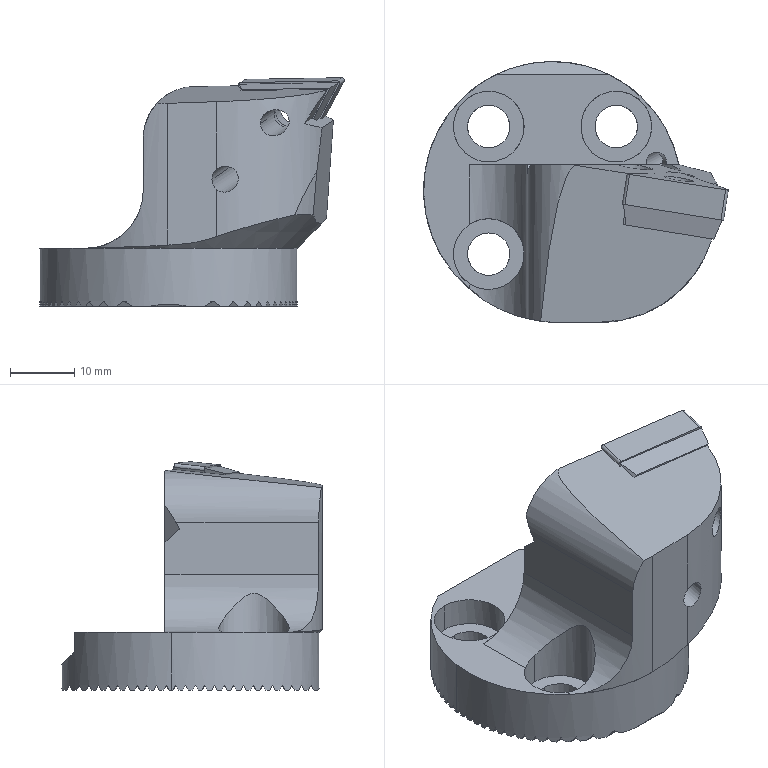NC program | Mastercam | posted with a generic post
Lines 8003 to 9736 of 11065, first 1620 of 1734 lines:
(4 FEMR |TOOL - 6|DIA. OFF. - 6|LEN. - 6|TOOL DIA. - 4.)
N6152 T6 M6
N6154 G0 G54 G90 X26.879 Y19.28 C9. B-84. S3500 M3
N6156 G43 H6 Z58.245
N6158 Z9.245
N6160 G1 Z8.146 F2000.
N6162 G41 D6 X26.556 Y19.863 F500.
N6164 G3 X26.468 Y19.915 I-.088 J-.049
N6166 X26.42 Y19.902 J-.101
N6168 G1 X25.334 Y19.3
N6170 X22.57 Y19.348
N6172 X22.567
N6174 G3 X22.437 Y19.218 J-.13
N6176 X22.565 Y19.088 I.13
N6178 G1 X25.33 Y19.04
N6180 X26.394 Y18.401
N6182 G3 X26.445 Y18.387 I.051 J.086
N6184 X26.531 Y18.435 J.1
N6186 G1 G40 X26.874 Y19.007
N6188 X26.879 Y19.28
N6190 Z8.046 F2000.
N6192 G41 D6 X26.556 Y19.863 F500.
N6194 G3 X26.468 Y19.915 I-.088 J-.049
N6196 X26.42 Y19.902 J-.101
N6198 G1 X25.334 Y19.3
N6200 X22.57 Y19.348
N6202 X22.567
N6204 G3 X22.437 Y19.218 J-.13
N6206 X22.565 Y19.088 I.13
N6208 G1 X25.33 Y19.04
N6210 X26.394 Y18.401
N6212 G3 X26.445 Y18.387 I.051 J.086
N6214 X26.531 Y18.435 J.1
N6216 G1 G40 X26.874 Y19.007
N6218 X26.879 Y19.28
N6220 Z7.947 F2000.
N6222 G41 D6 X26.556 Y19.863 F500.
N6224 G3 X26.468 Y19.915 I-.088 J-.049
N6226 X26.42 Y19.902 J-.101
N6228 G1 X25.334 Y19.3
N6230 X22.57 Y19.348
N6232 X22.567
N6234 G3 X22.437 Y19.218 J-.13
N6236 X22.565 Y19.088 I.13
N6238 G1 X25.33 Y19.04
N6240 X26.394 Y18.401
N6242 G3 X26.445 Y18.387 I.051 J.086
N6244 X26.531 Y18.435 J.1
N6246 G1 G40 X26.874 Y19.007
N6248 X26.879 Y19.28
N6250 Z7.848 F2000.
N6252 G41 D6 X26.556 Y19.863 F500.
N6254 G3 X26.468 Y19.915 I-.088 J-.049
N6256 X26.42 Y19.902 J-.101
N6258 G1 X25.334 Y19.3
N6260 X22.57 Y19.348
N6262 X22.567
N6264 G3 X22.437 Y19.218 J-.13
N6266 X22.565 Y19.088 I.13
N6268 G1 X25.33 Y19.04
N6270 X26.394 Y18.401
N6272 G3 X26.445 Y18.387 I.051 J.086
N6274 X26.531 Y18.435 J.1
N6276 G1 G40 X26.874 Y19.007
N6278 X26.879 Y19.28
N6280 Z7.748 F2000.
N6282 G41 D6 X26.556 Y19.863 F500.
N6284 G3 X26.468 Y19.915 I-.088 J-.049
N6286 X26.42 Y19.902 J-.101
N6288 G1 X25.334 Y19.3
N6290 X22.57 Y19.348
N6292 X22.567
N6294 G3 X22.437 Y19.218 J-.13
N6296 X22.565 Y19.088 I.13
N6298 G1 X25.33 Y19.04
N6300 X26.394 Y18.401
N6302 G3 X26.445 Y18.387 I.051 J.086
N6304 X26.531 Y18.435 J.1
N6306 G1 G40 X26.874 Y19.007
N6308 X26.879 Y19.28
N6310 Z7.649 F2000.
N6312 G41 D6 X26.556 Y19.863 F500.
N6314 G3 X26.468 Y19.915 I-.088 J-.049
N6316 X26.42 Y19.902 J-.101
N6318 G1 X25.334 Y19.3
N6320 X22.57 Y19.348
N6322 X22.567
N6324 G3 X22.437 Y19.218 J-.13
N6326 X22.565 Y19.088 I.13
N6328 G1 X25.33 Y19.04
N6330 X26.394 Y18.401
N6332 G3 X26.445 Y18.387 I.051 J.086
N6334 X26.531 Y18.435 J.1
N6336 G1 G40 X26.874 Y19.007
N6338 X26.879 Y19.28
N6340 Z7.55 F2000.
N6342 G41 D6 X26.556 Y19.863 F500.
N6344 G3 X26.468 Y19.915 I-.088 J-.049
N6346 X26.42 Y19.902 J-.101
N6348 G1 X25.334 Y19.3
N6350 X22.57 Y19.348
N6352 X22.567
N6354 G3 X22.437 Y19.218 J-.13
N6356 X22.565 Y19.088 I.13
N6358 G1 X25.33 Y19.04
N6360 X26.394 Y18.401
N6362 G3 X26.445 Y18.387 I.051 J.086
N6364 X26.531 Y18.435 J.1
N6366 G1 G40 X26.874 Y19.007
N6368 X26.879 Y19.28
N6370 Z7.45 F2000.
N6372 G41 D6 X26.556 Y19.863 F500.
N6374 G3 X26.468 Y19.915 I-.088 J-.049
N6376 X26.42 Y19.902 J-.101
N6378 G1 X25.334 Y19.3
N6380 X22.57 Y19.348
N6382 X22.567
N6384 G3 X22.437 Y19.218 J-.13
N6386 X22.565 Y19.088 I.13
N6388 G1 X25.33 Y19.04
N6390 X26.394 Y18.401
N6392 G3 X26.445 Y18.387 I.051 J.086
N6394 X26.531 Y18.435 J.1
N6396 G1 G40 X26.874 Y19.007
N6398 X26.879 Y19.28
N6400 Z7.351 F2000.
N6402 G41 D6 X26.556 Y19.863 F500.
N6404 G3 X26.468 Y19.915 I-.088 J-.049
N6406 X26.42 Y19.902 J-.101
N6408 G1 X25.334 Y19.3
N6410 X22.57 Y19.348
N6412 X22.567
N6414 G3 X22.437 Y19.218 J-.13
N6416 X22.565 Y19.088 I.13
N6418 G1 X25.33 Y19.04
N6420 X26.394 Y18.401
N6422 G3 X26.445 Y18.387 I.051 J.086
N6424 X26.531 Y18.435 J.1
N6426 G1 G40 X26.874 Y19.007
N6428 X26.879 Y19.28
N6430 Z7.251 F2000.
N6432 G41 D6 X26.556 Y19.863 F500.
N6434 G3 X26.468 Y19.915 I-.088 J-.049
N6436 X26.42 Y19.902 J-.101
N6438 G1 X25.334 Y19.3
N6440 X22.57 Y19.348
N6442 X22.567
N6444 G3 X22.437 Y19.218 J-.13
N6446 X22.565 Y19.088 I.13
N6448 G1 X25.33 Y19.04
N6450 X26.394 Y18.401
N6452 G3 X26.445 Y18.387 I.051 J.086
N6454 X26.531 Y18.435 J.1
N6456 G1 G40 X26.874 Y19.007
N6458 X26.879 Y19.28
N6460 Z7.152 F2000.
N6462 G41 D6 X26.556 Y19.863 F500.
N6464 G3 X26.468 Y19.915 I-.088 J-.049
N6466 X26.42 Y19.902 J-.101
N6468 G1 X25.334 Y19.3
N6470 X22.57 Y19.348
N6472 X22.567
N6474 G3 X22.437 Y19.218 J-.13
N6476 X22.565 Y19.088 I.13
N6478 G1 X25.33 Y19.04
N6480 X26.394 Y18.401
N6482 G3 X26.445 Y18.387 I.051 J.086
N6484 X26.531 Y18.435 J.1
N6486 G1 G40 X26.874 Y19.007
N6488 X26.879 Y19.28
N6490 Z7.053 F2000.
N6492 G41 D6 X26.556 Y19.863 F500.
N6494 G3 X26.468 Y19.915 I-.088 J-.049
N6496 X26.42 Y19.902 J-.101
N6498 G1 X25.334 Y19.3
N6500 X22.57 Y19.348
N6502 X22.567
N6504 G3 X22.437 Y19.218 J-.13
N6506 X22.565 Y19.088 I.13
N6508 G1 X25.33 Y19.04
N6510 X26.394 Y18.401
N6512 G3 X26.445 Y18.387 I.051 J.086
N6514 X26.531 Y18.435 J.1
N6516 G1 G40 X26.874 Y19.007
N6518 X26.879 Y19.28
N6520 Z6.953 F2000.
N6522 G41 D6 X26.556 Y19.863 F500.
N6524 G3 X26.468 Y19.915 I-.088 J-.049
N6526 X26.42 Y19.902 J-.101
N6528 G1 X25.334 Y19.3
N6530 X22.57 Y19.348
N6532 X22.567
N6534 G3 X22.437 Y19.218 J-.13
N6536 X22.565 Y19.088 I.13
N6538 G1 X25.33 Y19.04
N6540 X26.394 Y18.401
N6542 G3 X26.445 Y18.387 I.051 J.086
N6544 X26.531 Y18.435 J.1
N6546 G1 G40 X26.874 Y19.007
N6548 X26.879 Y19.28
N6550 Z6.854 F2000.
N6552 G41 D6 X26.556 Y19.863 F500.
N6554 G3 X26.468 Y19.915 I-.088 J-.049
N6556 X26.42 Y19.902 J-.101
N6558 G1 X25.334 Y19.3
N6560 X22.57 Y19.348
N6562 X22.567
N6564 G3 X22.437 Y19.218 J-.13
N6566 X22.565 Y19.088 I.13
N6568 G1 X25.33 Y19.04
N6570 X26.394 Y18.401
N6572 G3 X26.445 Y18.387 I.051 J.086
N6574 X26.531 Y18.435 J.1
N6576 G1 G40 X26.874 Y19.007
N6578 X26.879 Y19.28
N6580 Z6.754 F2000.
N6582 G41 D6 X26.556 Y19.863 F500.
N6584 G3 X26.468 Y19.915 I-.088 J-.049
N6586 X26.42 Y19.902 J-.101
N6588 G1 X25.334 Y19.3
N6590 X22.57 Y19.348
N6592 X22.567
N6594 G3 X22.437 Y19.218 J-.13
N6596 X22.565 Y19.088 I.13
N6598 G1 X25.33 Y19.04
N6600 X26.394 Y18.401
N6602 G3 X26.445 Y18.387 I.051 J.086
N6604 X26.531 Y18.435 J.1
N6606 G1 G40 X26.874 Y19.007
N6608 X26.879 Y19.28
N6610 Z6.655 F2000.
N6612 G41 D6 X26.556 Y19.863 F500.
N6614 G3 X26.468 Y19.915 I-.088 J-.049
N6616 X26.42 Y19.902 J-.101
N6618 G1 X25.334 Y19.3
N6620 X22.57 Y19.348
N6622 X22.567
N6624 G3 X22.437 Y19.218 J-.13
N6626 X22.565 Y19.088 I.13
N6628 G1 X25.33 Y19.04
N6630 X26.394 Y18.401
N6632 G3 X26.445 Y18.387 I.051 J.086
N6634 X26.531 Y18.435 J.1
N6636 G1 G40 X26.874 Y19.007
N6638 X26.879 Y19.28
N6640 Z6.556 F2000.
N6642 G41 D6 X26.556 Y19.863 F500.
N6644 G3 X26.468 Y19.915 I-.088 J-.049
N6646 X26.42 Y19.902 J-.101
N6648 G1 X25.334 Y19.3
N6650 X22.57 Y19.348
N6652 X22.567
N6654 G3 X22.437 Y19.218 J-.13
N6656 X22.565 Y19.088 I.13
N6658 G1 X25.33 Y19.04
N6660 X26.394 Y18.401
N6662 G3 X26.445 Y18.387 I.051 J.086
N6664 X26.531 Y18.435 J.1
N6666 G1 G40 X26.874 Y19.007
N6668 X26.879 Y19.28
N6670 Z6.456 F2000.
N6672 G41 D6 X26.556 Y19.863 F500.
N6674 G3 X26.468 Y19.915 I-.088 J-.049
N6676 X26.42 Y19.902 J-.101
N6678 G1 X25.334 Y19.3
N6680 X22.57 Y19.348
N6682 X22.567
N6684 G3 X22.437 Y19.218 J-.13
N6686 X22.565 Y19.088 I.13
N6688 G1 X25.33 Y19.04
N6690 X26.394 Y18.401
N6692 G3 X26.445 Y18.387 I.051 J.086
N6694 X26.531 Y18.435 J.1
N6696 G1 G40 X26.874 Y19.007
N6698 X26.879 Y19.28
N6700 Z6.357 F2000.
N6702 G41 D6 X26.556 Y19.863 F500.
N6704 G3 X26.468 Y19.915 I-.088 J-.049
N6706 X26.42 Y19.902 J-.101
N6708 G1 X25.334 Y19.3
N6710 X22.57 Y19.348
N6712 X22.567
N6714 G3 X22.437 Y19.218 J-.13
N6716 X22.565 Y19.088 I.13
N6718 G1 X25.33 Y19.04
N6720 X26.394 Y18.401
N6722 G3 X26.445 Y18.387 I.051 J.086
N6724 X26.531 Y18.435 J.1
N6726 G1 G40 X26.874 Y19.007
N6728 X26.879 Y19.28
N6730 Z6.257 F2000.
N6732 G41 D6 X26.556 Y19.863 F500.
N6734 G3 X26.468 Y19.915 I-.088 J-.049
N6736 X26.42 Y19.902 J-.101
N6738 G1 X25.334 Y19.3
N6740 X22.57 Y19.348
N6742 X22.567
N6744 G3 X22.437 Y19.218 J-.13
N6746 X22.565 Y19.088 I.13
N6748 G1 X25.33 Y19.04
N6750 X26.394 Y18.401
N6752 G3 X26.445 Y18.387 I.051 J.086
N6754 X26.531 Y18.435 J.1
N6756 G1 G40 X26.874 Y19.007
N6758 X26.879 Y19.28
N6760 Z6.158 F2000.
N6762 G41 D6 X26.556 Y19.863 F500.
N6764 G3 X26.468 Y19.915 I-.088 J-.049
N6766 X26.42 Y19.902 J-.101
N6768 G1 X25.334 Y19.3
N6770 X22.57 Y19.348
N6772 X22.567
N6774 G3 X22.437 Y19.218 J-.13
N6776 X22.565 Y19.088 I.13
N6778 G1 X25.33 Y19.04
N6780 X26.394 Y18.401
N6782 G3 X26.445 Y18.387 I.051 J.086
N6784 X26.531 Y18.435 J.1
N6786 G1 G40 X26.874 Y19.007
N6788 X26.879 Y19.28
N6790 Z6.059 F2000.
N6792 G41 D6 X26.556 Y19.863 F500.
N6794 G3 X26.468 Y19.915 I-.088 J-.049
N6796 X26.42 Y19.902 J-.101
N6798 G1 X25.334 Y19.3
N6800 X22.57 Y19.348
N6802 X22.567
N6804 G3 X22.437 Y19.218 J-.13
N6806 X22.565 Y19.088 I.13
N6808 G1 X25.33 Y19.04
N6810 X26.394 Y18.401
N6812 G3 X26.445 Y18.387 I.051 J.086
N6814 X26.531 Y18.435 J.1
N6816 G1 G40 X26.874 Y19.007
N6818 X26.879 Y19.28
N6820 Z5.959 F2000.
N6822 G41 D6 X26.556 Y19.863 F500.
N6824 G3 X26.468 Y19.915 I-.088 J-.049
N6826 X26.42 Y19.902 J-.101
N6828 G1 X25.334 Y19.3
N6830 X22.57 Y19.348
N6832 X22.567
N6834 G3 X22.437 Y19.218 J-.13
N6836 X22.565 Y19.088 I.13
N6838 G1 X25.33 Y19.04
N6840 X26.394 Y18.401
N6842 G3 X26.445 Y18.387 I.051 J.086
N6844 X26.531 Y18.435 J.1
N6846 G1 G40 X26.874 Y19.007
N6848 X26.879 Y19.28
N6850 Z5.86 F2000.
N6852 G41 D6 X26.556 Y19.863 F500.
N6854 G3 X26.468 Y19.915 I-.088 J-.049
N6856 X26.42 Y19.902 J-.101
N6858 G1 X25.334 Y19.3
N6860 X22.57 Y19.348
N6862 X22.567
N6864 G3 X22.437 Y19.218 J-.13
N6866 X22.565 Y19.088 I.13
N6868 G1 X25.33 Y19.04
N6870 X26.394 Y18.401
N6872 G3 X26.445 Y18.387 I.051 J.086
N6874 X26.531 Y18.435 J.1
N6876 G1 G40 X26.874 Y19.007
N6878 X26.879 Y19.28
N6880 Z5.76 F2000.
N6882 G41 D6 X26.556 Y19.863 F500.
N6884 G3 X26.468 Y19.915 I-.088 J-.049
N6886 X26.42 Y19.902 J-.101
N6888 G1 X25.334 Y19.3
N6890 X22.57 Y19.348
N6892 X22.567
N6894 G3 X22.437 Y19.218 J-.13
N6896 X22.565 Y19.088 I.13
N6898 G1 X25.33 Y19.04
N6900 X26.394 Y18.401
N6902 G3 X26.445 Y18.387 I.051 J.086
N6904 X26.531 Y18.435 J.1
N6906 G1 G40 X26.874 Y19.007
N6908 X26.879 Y19.28
N6910 Z5.661 F2000.
N6912 G41 D6 X26.556 Y19.863 F500.
N6914 G3 X26.468 Y19.915 I-.088 J-.049
N6916 X26.42 Y19.902 J-.101
N6918 G1 X25.334 Y19.3
N6920 X22.57 Y19.348
N6922 X22.567
N6924 G3 X22.437 Y19.218 J-.13
N6926 X22.565 Y19.088 I.13
N6928 G1 X25.33 Y19.04
N6930 X26.394 Y18.401
N6932 G3 X26.445 Y18.387 I.051 J.086
N6934 X26.531 Y18.435 J.1
N6936 G1 G40 X26.874 Y19.007
N6938 X26.879 Y19.28
N6940 Z5.562 F2000.
N6942 G41 D6 X26.556 Y19.863 F500.
N6944 G3 X26.468 Y19.915 I-.088 J-.049
N6946 X26.42 Y19.902 J-.101
N6948 G1 X25.334 Y19.3
N6950 X22.57 Y19.348
N6952 X22.567
N6954 G3 X22.437 Y19.218 J-.13
N6956 X22.565 Y19.088 I.13
N6958 G1 X25.33 Y19.04
N6960 X26.394 Y18.401
N6962 G3 X26.445 Y18.387 I.051 J.086
N6964 X26.531 Y18.435 J.1
N6966 G1 G40 X26.874 Y19.007
N6968 X26.879 Y19.28
N6970 Z5.462 F2000.
N6972 G41 D6 X26.556 Y19.863 F500.
N6974 G3 X26.468 Y19.915 I-.088 J-.049
N6976 X26.42 Y19.902 J-.101
N6978 G1 X25.334 Y19.3
N6980 X22.57 Y19.348
N6982 X22.567
N6984 G3 X22.437 Y19.218 J-.13
N6986 X22.565 Y19.088 I.13
N6988 G1 X25.33 Y19.04
N6990 X26.394 Y18.401
N6992 G3 X26.445 Y18.387 I.051 J.086
N6994 X26.531 Y18.435 J.1
N6996 G1 G40 X26.874 Y19.007
N6998 X26.879 Y19.28
N7000 Z5.363 F2000.
N7002 G41 D6 X26.556 Y19.863 F500.
N7004 G3 X26.468 Y19.915 I-.088 J-.049
N7006 X26.42 Y19.902 J-.101
N7008 G1 X25.334 Y19.3
N7010 X22.57 Y19.348
N7012 X22.567
N7014 G3 X22.437 Y19.218 J-.13
N7016 X22.565 Y19.088 I.13
N7018 G1 X25.33 Y19.04
N7020 X26.394 Y18.401
N7022 G3 X26.445 Y18.387 I.051 J.086
N7024 X26.531 Y18.435 J.1
N7026 G1 G40 X26.874 Y19.007
N7028 X26.879 Y19.28
N7030 Z5.263 F2000.
N7032 G41 D6 X26.556 Y19.863 F500.
N7034 G3 X26.468 Y19.915 I-.088 J-.049
N7036 X26.42 Y19.902 J-.101
N7038 G1 X25.334 Y19.3
N7040 X22.57 Y19.348
N7042 X22.567
N7044 G3 X22.437 Y19.218 J-.13
N7046 X22.565 Y19.088 I.13
N7048 G1 X25.33 Y19.04
N7050 X26.394 Y18.401
N7052 G3 X26.445 Y18.387 I.051 J.086
N7054 X26.531 Y18.435 J.1
N7056 G1 G40 X26.874 Y19.007
N7058 X26.879 Y19.28
N7060 Z5.164 F2000.
N7062 G41 D6 X26.556 Y19.863 F500.
N7064 G3 X26.468 Y19.915 I-.088 J-.049
N7066 X26.42 Y19.902 J-.101
N7068 G1 X25.334 Y19.3
N7070 X22.57 Y19.348
N7072 X22.567
N7074 G3 X22.437 Y19.218 J-.13
N7076 X22.565 Y19.088 I.13
N7078 G1 X25.33 Y19.04
N7080 X26.394 Y18.401
N7082 G3 X26.445 Y18.387 I.051 J.086
N7084 X26.531 Y18.435 J.1
N7086 G1 G40 X26.874 Y19.007
N7088 X26.879 Y19.28
N7090 Z5.065 F2000.
N7092 G41 D6 X26.556 Y19.863 F500.
N7094 G3 X26.468 Y19.915 I-.088 J-.049
N7096 X26.42 Y19.902 J-.101
N7098 G1 X25.334 Y19.3
N7100 X22.57 Y19.348
N7102 X22.567
N7104 G3 X22.437 Y19.218 J-.13
N7106 X22.565 Y19.088 I.13
N7108 G1 X25.33 Y19.04
N7110 X26.394 Y18.401
N7112 G3 X26.445 Y18.387 I.051 J.086
N7114 X26.531 Y18.435 J.1
N7116 G1 G40 X26.874 Y19.007
N7118 X26.879 Y19.28
N7120 Z4.965 F2000.
N7122 G41 D6 X26.556 Y19.863 F500.
N7124 G3 X26.468 Y19.915 I-.088 J-.049
N7126 X26.42 Y19.902 J-.101
N7128 G1 X25.334 Y19.3
N7130 X22.57 Y19.348
N7132 X22.567
N7134 G3 X22.437 Y19.218 J-.13
N7136 X22.565 Y19.088 I.13
N7138 G1 X25.33 Y19.04
N7140 X26.394 Y18.401
N7142 G3 X26.445 Y18.387 I.051 J.086
N7144 X26.531 Y18.435 J.1
N7146 G1 G40 X26.874 Y19.007
N7148 X26.879 Y19.28
N7150 Z4.866 F2000.
N7152 G41 D6 X26.556 Y19.863 F500.
N7154 G3 X26.468 Y19.915 I-.088 J-.049
N7156 X26.42 Y19.902 J-.101
N7158 G1 X25.334 Y19.3
N7160 X22.57 Y19.348
N7162 X22.567
N7164 G3 X22.437 Y19.218 J-.13
N7166 X22.565 Y19.088 I.13
N7168 G1 X25.33 Y19.04
N7170 X26.394 Y18.401
N7172 G3 X26.445 Y18.387 I.051 J.086
N7174 X26.531 Y18.435 J.1
N7176 G1 G40 X26.874 Y19.007
N7178 X26.879 Y19.28
N7180 Z4.766 F2000.
N7182 G41 D6 X26.556 Y19.863 F500.
N7184 G3 X26.468 Y19.915 I-.088 J-.049
N7186 X26.42 Y19.902 J-.101
N7188 G1 X25.334 Y19.3
N7190 X22.57 Y19.348
N7192 X22.567
N7194 G3 X22.437 Y19.218 J-.13
N7196 X22.565 Y19.088 I.13
N7198 G1 X25.33 Y19.04
N7200 X26.394 Y18.401
N7202 G3 X26.445 Y18.387 I.051 J.086
N7204 X26.531 Y18.435 J.1
N7206 G1 G40 X26.874 Y19.007
N7208 X26.879 Y19.28
N7210 Z4.667 F2000.
N7212 G41 D6 X26.556 Y19.863 F500.
N7214 G3 X26.468 Y19.915 I-.088 J-.049
N7216 X26.42 Y19.902 J-.101
N7218 G1 X25.334 Y19.3
N7220 X22.57 Y19.348
N7222 X22.567
N7224 G3 X22.437 Y19.218 J-.13
N7226 X22.565 Y19.088 I.13
N7228 G1 X25.33 Y19.04
N7230 X26.394 Y18.401
N7232 G3 X26.445 Y18.387 I.051 J.086
N7234 X26.531 Y18.435 J.1
N7236 G1 G40 X26.874 Y19.007
N7238 X26.879 Y19.28
N7240 Z4.568 F2000.
N7242 G41 D6 X26.556 Y19.863 F500.
N7244 G3 X26.468 Y19.915 I-.088 J-.049
N7246 X26.42 Y19.902 J-.101
N7248 G1 X25.334 Y19.3
N7250 X22.57 Y19.348
N7252 X22.567
N7254 G3 X22.437 Y19.218 J-.13
N7256 X22.565 Y19.088 I.13
N7258 G1 X25.33 Y19.04
N7260 X26.394 Y18.401
N7262 G3 X26.445 Y18.387 I.051 J.086
N7264 X26.531 Y18.435 J.1
N7266 G1 G40 X26.874 Y19.007
N7268 X26.879 Y19.28
N7270 Z4.468 F2000.
N7272 G41 D6 X26.556 Y19.863 F500.
N7274 G3 X26.468 Y19.915 I-.088 J-.049
N7276 X26.42 Y19.902 J-.101
N7278 G1 X25.334 Y19.3
N7280 X22.57 Y19.348
N7282 X22.567
N7284 G3 X22.437 Y19.218 J-.13
N7286 X22.565 Y19.088 I.13
N7288 G1 X25.33 Y19.04
N7290 X26.394 Y18.401
N7292 G3 X26.445 Y18.387 I.051 J.086
N7294 X26.531 Y18.435 J.1
N7296 G1 G40 X26.874 Y19.007
N7298 X26.879 Y19.28
N7300 Z4.369 F2000.
N7302 G41 D6 X26.556 Y19.863 F500.
N7304 G3 X26.468 Y19.915 I-.088 J-.049
N7306 X26.42 Y19.902 J-.101
N7308 G1 X25.334 Y19.3
N7310 X22.57 Y19.348
N7312 X22.567
N7314 G3 X22.437 Y19.218 J-.13
N7316 X22.565 Y19.088 I.13
N7318 G1 X25.33 Y19.04
N7320 X26.394 Y18.401
N7322 G3 X26.445 Y18.387 I.051 J.086
N7324 X26.531 Y18.435 J.1
N7326 G1 G40 X26.874 Y19.007
N7328 X26.879 Y19.28
N7330 Z4.269 F2000.
N7332 G41 D6 X26.556 Y19.863 F500.
N7334 G3 X26.468 Y19.915 I-.088 J-.049
N7336 X26.42 Y19.902 J-.101
N7338 G1 X25.334 Y19.3
N7340 X22.57 Y19.348
N7342 X22.567
N7344 G3 X22.437 Y19.218 J-.13
N7346 X22.565 Y19.088 I.13
N7348 G1 X25.33 Y19.04
N7350 X26.394 Y18.401
N7352 G3 X26.445 Y18.387 I.051 J.086
N7354 X26.531 Y18.435 J.1
N7356 G1 G40 X26.874 Y19.007
N7358 X26.879 Y19.28
N7360 Z4.17 F2000.
N7362 G41 D6 X26.556 Y19.863 F500.
N7364 G3 X26.468 Y19.915 I-.088 J-.049
N7366 X26.42 Y19.902 J-.101
N7368 G1 X25.334 Y19.3
N7370 X22.57 Y19.348
N7372 X22.567
N7374 G3 X22.437 Y19.218 J-.13
N7376 X22.565 Y19.088 I.13
N7378 G1 X25.33 Y19.04
N7380 X26.394 Y18.401
N7382 G3 X26.445 Y18.387 I.051 J.086
N7384 X26.531 Y18.435 J.1
N7386 G1 G40 X26.874 Y19.007
N7388 X26.879 Y19.28
N7390 Z4.071 F2000.
N7392 G41 D6 X26.556 Y19.863 F500.
N7394 G3 X26.468 Y19.915 I-.088 J-.049
N7396 X26.42 Y19.902 J-.101
N7398 G1 X25.334 Y19.3
N7400 X22.57 Y19.348
N7402 X22.567
N7404 G3 X22.437 Y19.218 J-.13
N7406 X22.565 Y19.088 I.13
N7408 G1 X25.33 Y19.04
N7410 X26.394 Y18.401
N7412 G3 X26.445 Y18.387 I.051 J.086
N7414 X26.531 Y18.435 J.1
N7416 G1 G40 X26.874 Y19.007
N7418 X26.879 Y19.28
N7420 Z3.971 F2000.
N7422 G41 D6 X26.556 Y19.863 F500.
N7424 G3 X26.468 Y19.915 I-.088 J-.049
N7426 X26.42 Y19.902 J-.101
N7428 G1 X25.334 Y19.3
N7430 X22.57 Y19.348
N7432 X22.567
N7434 G3 X22.437 Y19.218 J-.13
N7436 X22.565 Y19.088 I.13
N7438 G1 X25.33 Y19.04
N7440 X26.394 Y18.401
N7442 G3 X26.445 Y18.387 I.051 J.086
N7444 X26.531 Y18.435 J.1
N7446 G1 G40 X26.874 Y19.007
N7448 X26.879 Y19.28
N7450 Z3.872 F2000.
N7452 G41 D6 X26.556 Y19.863 F500.
N7454 G3 X26.468 Y19.915 I-.088 J-.049
N7456 X26.42 Y19.902 J-.101
N7458 G1 X25.334 Y19.3
N7460 X22.57 Y19.348
N7462 X22.567
N7464 G3 X22.437 Y19.218 J-.13
N7466 X22.565 Y19.088 I.13
N7468 G1 X25.33 Y19.04
N7470 X26.394 Y18.401
N7472 G3 X26.445 Y18.387 I.051 J.086
N7474 X26.531 Y18.435 J.1
N7476 G1 G40 X26.874 Y19.007
N7478 X26.879 Y19.28
N7480 Z3.772 F2000.
N7482 G41 D6 X26.556 Y19.863 F500.
N7484 G3 X26.468 Y19.915 I-.088 J-.049
N7486 X26.42 Y19.902 J-.101
N7488 G1 X25.334 Y19.3
N7490 X22.57 Y19.348
N7492 X22.567
N7494 G3 X22.437 Y19.218 J-.13
N7496 X22.565 Y19.088 I.13
N7498 G1 X25.33 Y19.04
N7500 X26.394 Y18.401
N7502 G3 X26.445 Y18.387 I.051 J.086
N7504 X26.531 Y18.435 J.1
N7506 G1 G40 X26.874 Y19.007
N7508 X26.879 Y19.28
N7510 Z3.673 F2000.
N7512 G41 D6 X26.556 Y19.863 F500.
N7514 G3 X26.468 Y19.915 I-.088 J-.049
N7516 X26.42 Y19.902 J-.101
N7518 G1 X25.334 Y19.3
N7520 X22.57 Y19.348
N7522 X22.567
N7524 G3 X22.437 Y19.218 J-.13
N7526 X22.565 Y19.088 I.13
N7528 G1 X25.33 Y19.04
N7530 X26.394 Y18.401
N7532 G3 X26.445 Y18.387 I.051 J.086
N7534 X26.531 Y18.435 J.1
N7536 G1 G40 X26.874 Y19.007
N7538 X26.879 Y19.28
N7540 Z3.574 F2000.
N7542 G41 D6 X26.556 Y19.863 F500.
N7544 G3 X26.468 Y19.915 I-.088 J-.049
N7546 X26.42 Y19.902 J-.101
N7548 G1 X25.334 Y19.3
N7550 X22.57 Y19.348
N7552 X22.567
N7554 G3 X22.437 Y19.218 J-.13
N7556 X22.565 Y19.088 I.13
N7558 G1 X25.33 Y19.04
N7560 X26.394 Y18.401
N7562 G3 X26.445 Y18.387 I.051 J.086
N7564 X26.531 Y18.435 J.1
N7566 G1 G40 X26.874 Y19.007
N7568 X26.879 Y19.28
N7570 Z3.474 F2000.
N7572 G41 D6 X26.556 Y19.863 F500.
N7574 G3 X26.468 Y19.915 I-.088 J-.049
N7576 X26.42 Y19.902 J-.101
N7578 G1 X25.334 Y19.3
N7580 X22.57 Y19.348
N7582 X22.567
N7584 G3 X22.437 Y19.218 J-.13
N7586 X22.565 Y19.088 I.13
N7588 G1 X25.33 Y19.04
N7590 X26.394 Y18.401
N7592 G3 X26.445 Y18.387 I.051 J.086
N7594 X26.531 Y18.435 J.1
N7596 G1 G40 X26.874 Y19.007
N7598 X26.879 Y19.28
N7600 Z3.375 F2000.
N7602 G41 D6 X26.556 Y19.863 F500.
N7604 G3 X26.468 Y19.915 I-.088 J-.049
N7606 X26.42 Y19.902 J-.101
N7608 G1 X25.334 Y19.3
N7610 X22.57 Y19.348
N7612 X22.567
N7614 G3 X22.437 Y19.218 J-.13
N7616 X22.565 Y19.088 I.13
N7618 G1 X25.33 Y19.04
N7620 X26.394 Y18.401
N7622 G3 X26.445 Y18.387 I.051 J.086
N7624 X26.531 Y18.435 J.1
N7626 G1 G40 X26.874 Y19.007
N7628 X26.879 Y19.28
N7630 Z3.275 F2000.
N7632 G41 D6 X26.556 Y19.863 F500.
N7634 G3 X26.468 Y19.915 I-.088 J-.049
N7636 X26.42 Y19.902 J-.101
N7638 G1 X25.334 Y19.3
N7640 X22.57 Y19.348
N7642 X22.567
N7644 G3 X22.437 Y19.218 J-.13
N7646 X22.565 Y19.088 I.13
N7648 G1 X25.33 Y19.04
N7650 X26.394 Y18.401
N7652 G3 X26.445 Y18.387 I.051 J.086
N7654 X26.531 Y18.435 J.1
N7656 G1 G40 X26.874 Y19.007
N7658 X26.879 Y19.28
N7660 Z3.176 F2000.
N7662 G41 D6 X26.556 Y19.863 F500.
N7664 G3 X26.468 Y19.915 I-.088 J-.049
N7666 X26.42 Y19.902 J-.101
N7668 G1 X25.334 Y19.3
N7670 X22.57 Y19.348
N7672 X22.567
N7674 G3 X22.437 Y19.218 J-.13
N7676 X22.565 Y19.088 I.13
N7678 G1 X25.33 Y19.04
N7680 X26.394 Y18.401
N7682 G3 X26.445 Y18.387 I.051 J.086
N7684 X26.531 Y18.435 J.1
N7686 G1 G40 X26.874 Y19.007
N7688 X26.879 Y19.28
N7690 Z3.077 F2000.
N7692 G41 D6 X26.556 Y19.863 F500.
N7694 G3 X26.468 Y19.915 I-.088 J-.049
N7696 X26.42 Y19.902 J-.101
N7698 G1 X25.334 Y19.3
N7700 X22.57 Y19.348
N7702 X22.567
N7704 G3 X22.437 Y19.218 J-.13
N7706 X22.565 Y19.088 I.13
N7708 G1 X25.33 Y19.04
N7710 X26.394 Y18.401
N7712 G3 X26.445 Y18.387 I.051 J.086
N7714 X26.531 Y18.435 J.1
N7716 G1 G40 X26.874 Y19.007
N7718 X26.879 Y19.28
N7720 Z2.977 F2000.
N7722 G41 D6 X26.556 Y19.863 F500.
N7724 G3 X26.468 Y19.915 I-.088 J-.049
N7726 X26.42 Y19.902 J-.101
N7728 G1 X25.334 Y19.3
N7730 X22.57 Y19.348
N7732 X22.567
N7734 G3 X22.437 Y19.218 J-.13
N7736 X22.565 Y19.088 I.13
N7738 G1 X25.33 Y19.04
N7740 X26.394 Y18.401
N7742 G3 X26.445 Y18.387 I.051 J.086
N7744 X26.531 Y18.435 J.1
N7746 G1 G40 X26.874 Y19.007
N7748 X26.879 Y19.28
N7750 Z2.878 F2000.
N7752 G41 D6 X26.556 Y19.863 F500.
N7754 G3 X26.468 Y19.915 I-.088 J-.049
N7756 X26.42 Y19.902 J-.101
N7758 G1 X25.334 Y19.3
N7760 X22.57 Y19.348
N7762 X22.567
N7764 G3 X22.437 Y19.218 J-.13
N7766 X22.565 Y19.088 I.13
N7768 G1 X25.33 Y19.04
N7770 X26.394 Y18.401
N7772 G3 X26.445 Y18.387 I.051 J.086
N7774 X26.531 Y18.435 J.1
N7776 G1 G40 X26.874 Y19.007
N7778 X26.879 Y19.28
N7780 Z2.778 F2000.
N7782 G41 D6 X26.556 Y19.863 F500.
N7784 G3 X26.468 Y19.915 I-.088 J-.049
N7786 X26.42 Y19.902 J-.101
N7788 G1 X25.334 Y19.3
N7790 X22.57 Y19.348
N7792 X22.567
N7794 G3 X22.437 Y19.218 J-.13
N7796 X22.565 Y19.088 I.13
N7798 G1 X25.33 Y19.04
N7800 X26.394 Y18.401
N7802 G3 X26.445 Y18.387 I.051 J.086
N7804 X26.531 Y18.435 J.1
N7806 G1 G40 X26.874 Y19.007
N7808 X26.879 Y19.28
N7810 Z2.679 F2000.
N7812 G41 D6 X26.556 Y19.863 F500.
N7814 G3 X26.468 Y19.915 I-.088 J-.049
N7816 X26.42 Y19.902 J-.101
N7818 G1 X25.334 Y19.3
N7820 X22.57 Y19.348
N7822 X22.567
N7824 G3 X22.437 Y19.218 J-.13
N7826 X22.565 Y19.088 I.13
N7828 G1 X25.33 Y19.04
N7830 X26.394 Y18.401
N7832 G3 X26.445 Y18.387 I.051 J.086
N7834 X26.531 Y18.435 J.1
N7836 G1 G40 X26.874 Y19.007
N7838 X26.879 Y19.28
N7840 Z2.58 F2000.
N7842 G41 D6 X26.556 Y19.863 F500.
N7844 G3 X26.468 Y19.915 I-.088 J-.049
N7846 X26.42 Y19.902 J-.101
N7848 G1 X25.334 Y19.3
N7850 X22.57 Y19.348
N7852 X22.567
N7854 G3 X22.437 Y19.218 J-.13
N7856 X22.565 Y19.088 I.13
N7858 G1 X25.33 Y19.04
N7860 X26.394 Y18.401
N7862 G3 X26.445 Y18.387 I.051 J.086
N7864 X26.531 Y18.435 J.1
N7866 G1 G40 X26.874 Y19.007
N7868 X26.879 Y19.28
N7870 Z2.48 F2000.
N7872 G41 D6 X26.556 Y19.863 F500.
N7874 G3 X26.468 Y19.915 I-.088 J-.049
N7876 X26.42 Y19.902 J-.101
N7878 G1 X25.334 Y19.3
N7880 X22.57 Y19.348
N7882 X22.567
N7884 G3 X22.437 Y19.218 J-.13
N7886 X22.565 Y19.088 I.13
N7888 G1 X25.33 Y19.04
N7890 X26.394 Y18.401
N7892 G3 X26.445 Y18.387 I.051 J.086
N7894 X26.531 Y18.435 J.1
N7896 G1 G40 X26.874 Y19.007
N7898 X26.879 Y19.28
N7900 Z2.381 F2000.
N7902 G41 D6 X26.556 Y19.863 F500.
N7904 G3 X26.468 Y19.915 I-.088 J-.049
N7906 X26.42 Y19.902 J-.101
N7908 G1 X25.334 Y19.3
N7910 X22.57 Y19.348
N7912 X22.567
N7914 G3 X22.437 Y19.218 J-.13
N7916 X22.565 Y19.088 I.13
N7918 G1 X25.33 Y19.04
N7920 X26.394 Y18.401
N7922 G3 X26.445 Y18.387 I.051 J.086
N7924 X26.531 Y18.435 J.1
N7926 G1 G40 X26.874 Y19.007
N7928 X26.879 Y19.28
N7930 Z2.281 F2000.
N7932 G41 D6 X26.556 Y19.863 F500.
N7934 G3 X26.468 Y19.915 I-.088 J-.049
N7936 X26.42 Y19.902 J-.101
N7938 G1 X25.334 Y19.3
N7940 X22.57 Y19.348
N7942 X22.567
N7944 G3 X22.437 Y19.218 J-.13
N7946 X22.565 Y19.088 I.13
N7948 G1 X25.33 Y19.04
N7950 X26.394 Y18.401
N7952 G3 X26.445 Y18.387 I.051 J.086
N7954 X26.531 Y18.435 J.1
N7956 G1 G40 X26.874 Y19.007
N7958 X26.879 Y19.28
N7960 Z2.182 F2000.
N7962 G41 D6 X26.556 Y19.863 F500.
N7964 G3 X26.468 Y19.915 I-.088 J-.049
N7966 X26.42 Y19.902 J-.101
N7968 G1 X25.334 Y19.3
N7970 X22.57 Y19.348
N7972 X22.567
N7974 G3 X22.437 Y19.218 J-.13
N7976 X22.565 Y19.088 I.13
N7978 G1 X25.33 Y19.04
N7980 X26.394 Y18.401
N7982 G3 X26.445 Y18.387 I.051 J.086
N7984 X26.531 Y18.435 J.1
N7986 G1 G40 X26.874 Y19.007
N7988 X26.879 Y19.28
N7990 Z2.083 F2000.
N7992 G41 D6 X26.556 Y19.863 F500.
N7994 G3 X26.468 Y19.915 I-.088 J-.049
N7996 X26.42 Y19.902 J-.101
N7998 G1 X25.334 Y19.3
N8000 X22.57 Y19.348
N8002 X22.567
N8004 G3 X22.437 Y19.218 J-.13
N8006 X22.565 Y19.088 I.13
N8008 G1 X25.33 Y19.04
N8010 X26.394 Y18.401
N8012 G3 X26.445 Y18.387 I.051 J.086
N8014 X26.531 Y18.435 J.1
N8016 G1 G40 X26.874 Y19.007
N8018 X26.879 Y19.28
N8020 Z1.983 F2000.
N8022 G41 D6 X26.556 Y19.863 F500.
N8024 G3 X26.468 Y19.915 I-.088 J-.049
N8026 X26.42 Y19.902 J-.101
N8028 G1 X25.334 Y19.3
N8030 X22.57 Y19.348
N8032 X22.567
N8034 G3 X22.437 Y19.218 J-.13
N8036 X22.565 Y19.088 I.13
N8038 G1 X25.33 Y19.04
N8040 X26.394 Y18.401
N8042 G3 X26.445 Y18.387 I.051 J.086
N8044 X26.531 Y18.435 J.1
N8046 G1 G40 X26.874 Y19.007
N8048 X26.879 Y19.28
N8050 Z1.884 F2000.
N8052 G41 D6 X26.556 Y19.863 F500.
N8054 G3 X26.468 Y19.915 I-.088 J-.049
N8056 X26.42 Y19.902 J-.101
N8058 G1 X25.334 Y19.3
N8060 X22.57 Y19.348
N8062 X22.567
N8064 G3 X22.437 Y19.218 J-.13
N8066 X22.565 Y19.088 I.13
N8068 G1 X25.33 Y19.04
N8070 X26.394 Y18.401
N8072 G3 X26.445 Y18.387 I.051 J.086
N8074 X26.531 Y18.435 J.1
N8076 G1 G40 X26.874 Y19.007
N8078 X26.879 Y19.28
N8080 Z1.784 F2000.
N8082 G41 D6 X26.556 Y19.863 F500.
N8084 G3 X26.468 Y19.915 I-.088 J-.049
N8086 X26.42 Y19.902 J-.101
N8088 G1 X25.334 Y19.3
N8090 X22.57 Y19.348
N8092 X22.567
N8094 G3 X22.437 Y19.218 J-.13
N8096 X22.565 Y19.088 I.13
N8098 G1 X25.33 Y19.04
N8100 X26.394 Y18.401
N8102 G3 X26.445 Y18.387 I.051 J.086
N8104 X26.531 Y18.435 J.1
N8106 G1 G40 X26.874 Y19.007
N8108 X26.879 Y19.28
N8110 Z1.685 F2000.
N8112 G41 D6 X26.556 Y19.863 F500.
N8114 G3 X26.468 Y19.915 I-.088 J-.049
N8116 X26.42 Y19.902 J-.101
N8118 G1 X25.334 Y19.3
N8120 X22.57 Y19.348
N8122 X22.567
N8124 G3 X22.437 Y19.218 J-.13
N8126 X22.565 Y19.088 I.13
N8128 G1 X25.33 Y19.04
N8130 X26.394 Y18.401
N8132 G3 X26.445 Y18.387 I.051 J.086
N8134 X26.531 Y18.435 J.1
N8136 G1 G40 X26.874 Y19.007
N8138 X26.879 Y19.28
N8140 Z1.586 F2000.
N8142 G41 D6 X26.556 Y19.863 F500.
N8144 G3 X26.468 Y19.915 I-.088 J-.049
N8146 X26.42 Y19.902 J-.101
N8148 G1 X25.334 Y19.3
N8150 X22.57 Y19.348
N8152 X22.567
N8154 G3 X22.437 Y19.218 J-.13
N8156 X22.565 Y19.088 I.13
N8158 G1 X25.33 Y19.04
N8160 X26.394 Y18.401
N8162 G3 X26.445 Y18.387 I.051 J.086
N8164 X26.531 Y18.435 J.1
N8166 G1 G40 X26.874 Y19.007
N8168 X26.879 Y19.28
N8170 Z1.486 F2000.
N8172 G41 D6 X26.556 Y19.863 F500.
N8174 G3 X26.468 Y19.915 I-.088 J-.049
N8176 X26.42 Y19.902 J-.101
N8178 G1 X25.334 Y19.3
N8180 X22.57 Y19.348
N8182 X22.567
N8184 G3 X22.437 Y19.218 J-.13
N8186 X22.565 Y19.088 I.13
N8188 G1 X25.33 Y19.04
N8190 X26.394 Y18.401
N8192 G3 X26.445 Y18.387 I.051 J.086
N8194 X26.531 Y18.435 J.1
N8196 G1 G40 X26.874 Y19.007
N8198 X26.879 Y19.28
N8200 Z1.387 F2000.
N8202 G41 D6 X26.556 Y19.863 F500.
N8204 G3 X26.468 Y19.915 I-.088 J-.049
N8206 X26.42 Y19.902 J-.101
N8208 G1 X25.334 Y19.3
N8210 X22.57 Y19.348
N8212 X22.567
N8214 G3 X22.437 Y19.218 J-.13
N8216 X22.565 Y19.088 I.13
N8218 G1 X25.33 Y19.04
N8220 X26.394 Y18.401
N8222 G3 X26.445 Y18.387 I.051 J.086
N8224 X26.531 Y18.435 J.1
N8226 G1 G40 X26.874 Y19.007
N8228 X26.879 Y19.28
N8230 Z1.287 F2000.
N8232 G41 D6 X26.556 Y19.863 F500.
N8234 G3 X26.468 Y19.915 I-.088 J-.049
N8236 X26.42 Y19.902 J-.101
N8238 G1 X25.334 Y19.3
N8240 X22.57 Y19.348
N8242 X22.567
N8244 G3 X22.437 Y19.218 J-.13
N8246 X22.565 Y19.088 I.13
N8248 G1 X25.33 Y19.04
N8250 X26.394 Y18.401
N8252 G3 X26.445 Y18.387 I.051 J.086
N8254 X26.531 Y18.435 J.1
N8256 G1 G40 X26.874 Y19.007
N8258 X26.879 Y19.28
N8260 Z1.188 F2000.
N8262 G41 D6 X26.556 Y19.863 F500.
N8264 G3 X26.468 Y19.915 I-.088 J-.049
N8266 X26.42 Y19.902 J-.101
N8268 G1 X25.334 Y19.3
N8270 X22.57 Y19.348
N8272 X22.567
N8274 G3 X22.437 Y19.218 J-.13
N8276 X22.565 Y19.088 I.13
N8278 G1 X25.33 Y19.04
N8280 X26.394 Y18.401
N8282 G3 X26.445 Y18.387 I.051 J.086
N8284 X26.531 Y18.435 J.1
N8286 G1 G40 X26.874 Y19.007
N8288 X26.879 Y19.28
N8290 Z1.089 F2000.
N8292 G41 D6 X26.556 Y19.863 F500.
N8294 G3 X26.468 Y19.915 I-.088 J-.049
N8296 X26.42 Y19.902 J-.101
N8298 G1 X25.334 Y19.3
N8300 X22.57 Y19.348
N8302 X22.567
N8304 G3 X22.437 Y19.218 J-.13
N8306 X22.565 Y19.088 I.13
N8308 G1 X25.33 Y19.04
N8310 X26.394 Y18.401
N8312 G3 X26.445 Y18.387 I.051 J.086
N8314 X26.531 Y18.435 J.1
N8316 G1 G40 X26.874 Y19.007
N8318 X26.879 Y19.28
N8320 Z.989 F2000.
N8322 G41 D6 X26.556 Y19.863 F500.
N8324 G3 X26.468 Y19.915 I-.088 J-.049
N8326 X26.42 Y19.902 J-.101
N8328 G1 X25.334 Y19.3
N8330 X22.57 Y19.348
N8332 X22.567
N8334 G3 X22.437 Y19.218 J-.13
N8336 X22.565 Y19.088 I.13
N8338 G1 X25.33 Y19.04
N8340 X26.394 Y18.401
N8342 G3 X26.445 Y18.387 I.051 J.086
N8344 X26.531 Y18.435 J.1
N8346 G1 G40 X26.874 Y19.007
N8348 X26.879 Y19.28
N8350 Z.89 F2000.
N8352 G41 D6 X26.556 Y19.863 F500.
N8354 G3 X26.468 Y19.915 I-.088 J-.049
N8356 X26.42 Y19.902 J-.101
N8358 G1 X25.334 Y19.3
N8360 X22.57 Y19.348
N8362 X22.567
N8364 G3 X22.437 Y19.218 J-.13
N8366 X22.565 Y19.088 I.13
N8368 G1 X25.33 Y19.04
N8370 X26.394 Y18.401
N8372 G3 X26.445 Y18.387 I.051 J.086
N8374 X26.531 Y18.435 J.1
N8376 G1 G40 X26.874 Y19.007
N8378 X26.879 Y19.28
N8380 Z.79 F2000.
N8382 G41 D6 X26.556 Y19.863 F500.
N8384 G3 X26.468 Y19.915 I-.088 J-.049
N8386 X26.42 Y19.902 J-.101
N8388 G1 X25.334 Y19.3
N8390 X22.57 Y19.348
N8392 X22.567
N8394 G3 X22.437 Y19.218 J-.13
N8396 X22.565 Y19.088 I.13
N8398 G1 X25.33 Y19.04
N8400 X26.394 Y18.401
N8402 G3 X26.445 Y18.387 I.051 J.086
N8404 X26.531 Y18.435 J.1
N8406 G1 G40 X26.874 Y19.007
N8408 X26.879 Y19.28
N8410 Z.691 F2000.
N8412 G41 D6 X26.556 Y19.863 F500.
N8414 G3 X26.468 Y19.915 I-.088 J-.049
N8416 X26.42 Y19.902 J-.101
N8418 G1 X25.334 Y19.3
N8420 X22.57 Y19.348
N8422 X22.567
N8424 G3 X22.437 Y19.218 J-.13
N8426 X22.565 Y19.088 I.13
N8428 G1 X25.33 Y19.04
N8430 X26.394 Y18.401
N8432 G3 X26.445 Y18.387 I.051 J.086
N8434 X26.531 Y18.435 J.1
N8436 G1 G40 X26.874 Y19.007
N8438 X26.879 Y19.28
N8440 Z.592 F2000.
N8442 G41 D6 X26.556 Y19.863 F500.
N8444 G3 X26.468 Y19.915 I-.088 J-.049
N8446 X26.42 Y19.902 J-.101
N8448 G1 X25.334 Y19.3
N8450 X22.57 Y19.348
N8452 X22.567
N8454 G3 X22.437 Y19.218 J-.13
N8456 X22.565 Y19.088 I.13
N8458 G1 X25.33 Y19.04
N8460 X26.394 Y18.401
N8462 G3 X26.445 Y18.387 I.051 J.086
N8464 X26.531 Y18.435 J.1
N8466 G1 G40 X26.874 Y19.007
N8468 X26.879 Y19.28
N8470 Z.492 F2000.
N8472 G41 D6 X26.556 Y19.863 F500.
N8474 G3 X26.468 Y19.915 I-.088 J-.049
N8476 X26.42 Y19.902 J-.101
N8478 G1 X25.334 Y19.3
N8480 X22.57 Y19.348
N8482 X22.567
N8484 G3 X22.437 Y19.218 J-.13
N8486 X22.565 Y19.088 I.13
N8488 G1 X25.33 Y19.04
N8490 X26.394 Y18.401
N8492 G3 X26.445 Y18.387 I.051 J.086
N8494 X26.531 Y18.435 J.1
N8496 G1 G40 X26.874 Y19.007
N8498 X26.879 Y19.28
N8500 Z.393 F2000.
N8502 G41 D6 X26.556 Y19.863 F500.
N8504 G3 X26.468 Y19.915 I-.088 J-.049
N8506 X26.42 Y19.902 J-.101
N8508 G1 X25.334 Y19.3
N8510 X22.57 Y19.348
N8512 X22.567
N8514 G3 X22.437 Y19.218 J-.13
N8516 X22.565 Y19.088 I.13
N8518 G1 X25.33 Y19.04
N8520 X26.394 Y18.401
N8522 G3 X26.445 Y18.387 I.051 J.086
N8524 X26.531 Y18.435 J.1
N8526 G1 G40 X26.874 Y19.007
N8528 X26.879 Y19.28
N8530 Z.293 F2000.
N8532 G41 D6 X26.556 Y19.863 F500.
N8534 G3 X26.468 Y19.915 I-.088 J-.049
N8536 X26.42 Y19.902 J-.101
N8538 G1 X25.334 Y19.3
N8540 X22.57 Y19.348
N8542 X22.567
N8544 G3 X22.437 Y19.218 J-.13
N8546 X22.565 Y19.088 I.13
N8548 G1 X25.33 Y19.04
N8550 X26.394 Y18.401
N8552 G3 X26.445 Y18.387 I.051 J.086
N8554 X26.531 Y18.435 J.1
N8556 G1 G40 X26.874 Y19.007
N8558 X26.879 Y19.28
N8560 Z.194 F2000.
N8562 G41 D6 X26.556 Y19.863 F500.
N8564 G3 X26.468 Y19.915 I-.088 J-.049
N8566 X26.42 Y19.902 J-.101
N8568 G1 X25.334 Y19.3
N8570 X22.57 Y19.348
N8572 X22.567
N8574 G3 X22.437 Y19.218 J-.13
N8576 X22.565 Y19.088 I.13
N8578 G1 X25.33 Y19.04
N8580 X26.394 Y18.401
N8582 G3 X26.445 Y18.387 I.051 J.086
N8584 X26.531 Y18.435 J.1
N8586 G1 G40 X26.874 Y19.007
N8588 X26.879 Y19.28
N8590 Z.095 F2000.
N8592 G41 D6 X26.556 Y19.863 F500.
N8594 G3 X26.468 Y19.915 I-.088 J-.049
N8596 X26.42 Y19.902 J-.101
N8598 G1 X25.334 Y19.3
N8600 X22.57 Y19.348
N8602 X22.567
N8604 G3 X22.437 Y19.218 J-.13
N8606 X22.565 Y19.088 I.13
N8608 G1 X25.33 Y19.04
N8610 X26.394 Y18.401
N8612 G3 X26.445 Y18.387 I.051 J.086
N8614 X26.531 Y18.435 J.1
N8616 G1 G40 X26.874 Y19.007
N8618 X26.879 Y19.28
N8620 Z-.005 F2000.
N8622 G41 D6 X26.556 Y19.863 F500.
N8624 G3 X26.468 Y19.915 I-.088 J-.049
N8626 X26.42 Y19.902 J-.101
N8628 G1 X25.334 Y19.3
N8630 X22.57 Y19.348
N8632 X22.567
N8634 G3 X22.437 Y19.218 J-.13
N8636 X22.565 Y19.088 I.13
N8638 G1 X25.33 Y19.04
N8640 X26.394 Y18.401
N8642 G3 X26.445 Y18.387 I.051 J.086
N8644 X26.531 Y18.435 J.1
N8646 G1 G40 X26.874 Y19.007
N8648 G0 Z58.245
N8650 Z61.48
N8652 X32.492 Y23.634
N8654 Z12.48
N8656 G1 Z3.23 F2000.
N8658 G41 D6 X29.868 Y22.179 F500.
N8660 X24.782 Y19.36
N8662 X22.571 Y19.398
N8664 X22.567
N8666 G3 X22.387 Y19.218 J-.18
N8668 X22.564 Y19.038 I.18
N8670 G1 X24.776 Y19.
N8672 X34.637 Y13.075
N8674 G40 X37.209 Y11.529
N8676 G0 Z61.48
N8678 M5
N8680 G0 G28 G91 Z0.
N8682 G28 C0. B0.
N8684 M01
N8686 G0 G17 G40 G80 G90 G94 G98
N8688 G0 G28 G91 Z0.
(12 FEMF |TOOL - 9|DIA. OFF. - 9|LEN. - 9|TOOL DIA. - 12.)
N8690 T9 M6
N8692 G0 G54 G90 X33.237 Y6.761 C0. B0. S3500 M3
N8694 G43 H9 Z90.239
N8696 Z11.239
N8698 G1 Z8.239 F2000.
N8700 G41 D9 X32.611 Y2.81 F600.
N8702 X31.175 Y-6.254
N8704 G2 X7.471 Y-26.5 I-23.704 J3.754
N8706 G1 X-.264
N8708 G2 X-16.83 Y-19.949 I1.479 J27.961
N8710 G1 G40 X-18.36 Y-18.66
N8712 G0 Z90.239
N8714 B-90.
N8716 X15. Y34.
N8718 Z54.7
N8720 Z5.7
N8722 G1 Z4.7 F2000.
N8724 G41 D9 Y25. F600.
N8726 Y-25.
N8728 G40 Y-34.
N8730 G0 Z54.7
N8732 M8
N8734 Z68.
N8736 X11.95 Y17.718
N8738 Z19.
N8740 G1 Z18. F2000.
N8742 G41 D9 Y8.718 F600.
N8744 Y-8.718
N8746 G40 Y-17.718
N8748 G0 Z68.
N8750 C9. B-84.
N8752 X11.13 Y34.98
N8754 Z47.905
N8756 Z-1.095
N8758 G1 Z-7.095 F2000.
N8760 G41 D9 X11.566 Y29.999 F600.
N8762 G3 X11.865 Y29.725 I.299 J.026
N8764 X11.891 Y29.726 J.3
N8766 G1 X12.389 Y29.77
N8768 X27.708 Y31.11
N8770 X28.206 Y31.154
N8772 G3 X28.48 Y31.453 I-.026 J.299
N8774 X28.479 Y31.479 I-.3
N8776 G1 G40 X28.043 Y36.46
N8778 G0 Z47.905
N8780 M9
N8782 Z76.5
N8784 X-15. Y-27.
N8786 C0. B-270.
N8788 Z-2.5
N8790 G1 Z-6.5 F2000.
N8792 G41 D9 Y-25. F600.
N8794 Y-12.899
N8796 G3 X-18. Y-9.899 I-3.
N8798 G1 X-26.101
N8800 G2 X-40.099 Y3.855 J14.
N8802 G1 X-40.508 Y27.126
N8804 X-40.526 Y28.126
N8806 G3 X-40.532 Y28.16 I-.099 J-.002
N8808 G1 G40 X-41.966 Y31.894
N8810 G0 Z76.5
N8812 C9. B-84.
N8814 X39.962 Y32.235
N8816 Z63.905
N8818 Z-15.095
N8820 G1 Z-18.095 F2000.
N8822 G41 D9 X39.858 Y26.236 F600.
N8824 X39.403 Y.214
N8826 G40 X39.299 Y-5.785
N8828 G0 Z63.905
N8830 M8
N8832 Z67.971
N8834 X-14.475 Y-17.718
N8836 C0. B-45.
N8838 Z18.971
N8840 G1 Z16.971 F2000.
N8842 G41 D9 Y-8.718 F600.
N8844 Y8.718
N8846 G40 Y17.718
N8848 G0 Z67.971
N8850 M9
N8852 C-70.321 B29.561
N8854 X8.518 Y17.139
N8856 Z66.876
N8858 Z36.876
N8860 G1 G41 D9 X10.001 Y10.298
N8862 X13.322 Y-5.02
N8864 G40 X14.805 Y-11.861
N8866 G0 Z66.876
N8868 M5
N8870 G0 G28 G91 Z0.
N8872 G28 C0. B0.
N8874 M01
N8876 G0 G17 G40 G80 G90 G94 G98
N8878 G0 G28 G91 Z0.
(30 INC |TOOL - 10|DIA. OFF. - 10|LEN. - 10|TOOL DIA. - 30.)
N8880 T10 M6
N8882 G0 G54 G90 X24. Y43. C0. B-90. S3500 M3
N8884 G43 H10 Z54.95
N8886 Z5.95
N8888 G1 Z3.95 F2000.
N8890 G41 D10 Y25. F400.
N8892 Y-25.
N8894 G40 Y-43.
N8896 G0 Z54.95
N8898 Z66.205
N8900 X27.066 Y42.566
N8902 C9. B-84.
N8904 Z17.205
N8906 G1 Z7.905 F2000.
N8908 G41 D10 X22.408 Y23.116 F600.
N8910 G3 X22.405 Y23.092 I.097 J-.024
N8912 X22.41 Y23.064 I.1
N8914 G1 X30.944 Y-5.686
N8916 G40 X33.789 Y-15.273
N8918 G0 Z66.205
N8920 M5
N8922 G0 G28 G91 Z0.
N8924 G28 C0. B0.
N8926 M01
N8928 G0 G17 G40 G80 G90 G94 G98
N8930 G0 G28 G91 Z0.
(6 CHM |TOOL - 12|DIA. OFF. - 12|LEN. - 12|TOOL DIA. - 6.)
N8932 T12 M6
N8934 G0 G54 G90 X18.229 Y8.796 C9. B-84. S2000 M3
N8936 G43 H12 Z57.468 M8
N8938 G81 G98 Z6.668 R8.468 F100.
N8940 G80
N8942 Z57.905
N8944 X21.594 Y11.867
N8946 G81 G98 Z7.105 R8.905 F100.
N8948 G80
N8950 X29.951 Y19.09
N8952 Z49.945
N8954 G81 G98 Z-.855 R.945 F100.
N8956 G80
N8958 M9
N8960 M5
N8962 G0 G28 G91 Z0.
N8964 G28 C0. B0.
N8966 M01
N8968 G0 G17 G40 G80 G90 G94 G98
N8970 G0 G28 G91 Z0.
(6 DR |TOOL - 3|DIA. OFF. - 3|LEN. - 3|TOOL DIA. - 6.)
N8972 T3 M6
N8974 G0 G54 G90 X21.594 Y11.867 C9. B-84. S2500 M3
N8976 G43 H3 Z57.905 M8
N8978 G81 G98 Z2.105 R8.905 F100.
N8980 G80
N8982 M9
N8984 M5
N8986 G0 G28 G91 Z0.
N8988 G28 C0. B0.
N8990 M01
N8992 G0 G17 G40 G80 G90 G94 G98
N8994 G0 G28 G91 Z0.
(3.3 DR |TOOL - 13|DIA. OFF. - 13|LEN. - 13|TOOL DIA. - 3.3)
N8996 T13 M6
N8998 G0 G54 G90 X29.951 Y19.09 C9. B-84. S2500 M3
N9000 G43 H13 Z49.945 M8
N9002 G83 G98 Z-13.055 R.945 Q2. F60.
N9004 G80
N9006 Z54.905
N9008 X21.594 Y11.867
N9010 G83 G98 Z-19.095 R5.905 Q2. F60.
N9012 G80
N9014 M9
N9016 M5
N9018 G0 G28 G91 Z0.
N9020 G28 C0. B0.
N9022 M01
N9024 G0 G17 G40 G80 G90 G94 G98
N9026 G0 G28 G91 Z0.
(6 CHM |TOOL - 12|DIA. OFF. - 12|LEN. - 12|TOOL DIA. - 6.)
M0
N9028 T12 M6
N9030 G0 G54 G90 X29.951 Y19.09 C9. B-84. S2000 M3
N9032 G43 H12 Z49.945 M8
N9034 G81 G98 Z-2.255 R.945 F100.
N9036 G80
N9038 M9
N9040 M5
N9042 G0 G28 G91 Z0.
N9044 G28 C0. B0.
N9046 M01
N9048 G0 G17 G40 G80 G90 G94 G98
N9050 G0 G28 G91 Z0.
(4.5 FEM |TOOL - 11|DIA. OFF. - 11|LEN. - 11|TOOL DIA. - 4.5)
N9052 T11 M6
N9054 G0 G54 G90 X29.951 Y-19.09 C189. B-96. S2000 M3
N9056 G43 H11 Z63.644
N9058 G81 G98 Z8.644 R14.644 F100.
N9060 G80
N9062 Z67.092
N9064 X21.594 Y-11.867
N9066 G83 G98 Z7.092 R18.092 Q2. F100.
N9068 G80
N9070 M5
N9072 G0 G28 G91 Z0.
N9074 G28 C0. B0.
N9076 M01
N9078 G0 G17 G40 G80 G90 G94 G98
N9080 G0 G28 G91 Z0.
(M4 XXXXXX |TOOL - 14|DIA. OFF. - 14|LEN. - 14|TOOL DIA. - 3.15)
N9082 T14 M6
N9084 G0 G54 G90 X29.951 Y19.09 C9. B-84. S2500 M3
N9086 G43 H14 Z49.945 M8
N9088 Z1.945
N9090 G1 Z-9.055 F600.
N9092 G41 D14 X30.176 F100.
N9094 G3 X29.951 Y19.315 Z-8.88 I-.225
N9096 X29.726 Y19.09 Z-8.705 J-.225
N9098 X29.951 Y18.865 Z-8.53 I.225
N9100 X30.176 Y19.09 Z-8.355 J.225
N9102 X29.951 Y19.315 Z-8.18 I-.225
N9104 X29.726 Y19.09 Z-8.005 J-.225
N9106 G1 G40 X29.951
N9108 Z-6.955 F600.
N9110 G41 D14 X30.176 F100.
N9112 G3 X29.951 Y19.315 Z-6.78 I-.225
N9114 X29.726 Y19.09 Z-6.605 J-.225
N9116 X29.951 Y18.865 Z-6.43 I.225
N9118 X30.176 Y19.09 Z-6.255 J.225
N9120 X29.951 Y19.315 Z-6.08 I-.225
N9122 X29.726 Y19.09 Z-5.905 J-.225
N9124 G1 G40 X29.951
N9126 Z-4.855 F600.
N9128 G41 D14 X30.176 F100.
N9130 G3 X29.951 Y19.315 Z-4.68 I-.225
N9132 X29.726 Y19.09 Z-4.505 J-.225
N9134 X29.951 Y18.865 Z-4.33 I.225
N9136 X30.176 Y19.09 Z-4.155 J.225
N9138 X29.951 Y19.315 Z-3.98 I-.225
N9140 X29.726 Y19.09 Z-3.805 J-.225
N9142 G1 G40 X29.951
N9144 Z-2.755 F600.
N9146 G41 D14 X30.176 F100.
N9148 G3 X29.951 Y19.315 Z-2.58 I-.225
N9150 X29.726 Y19.09 Z-2.405 J-.225
N9152 X29.951 Y18.865 Z-2.23 I.225
N9154 X30.176 Y19.09 Z-2.055 J.225
N9156 X29.951 Y19.315 Z-1.88 I-.225
N9158 X29.726 Y19.09 Z-1.705 J-.225
N9160 G1 G40 X29.951
N9162 Z-9.055 F600.
N9164 G41 D14 X30.276 F100.
N9166 G3 X29.951 Y19.415 Z-8.88 I-.325
N9168 X29.626 Y19.09 Z-8.705 J-.325
N9170 X29.951 Y18.765 Z-8.53 I.325
N9172 X30.276 Y19.09 Z-8.355 J.325
N9174 X29.951 Y19.415 Z-8.18 I-.325
N9176 X29.626 Y19.09 Z-8.005 J-.325
N9178 G1 G40 X29.951
N9180 Z-6.955 F600.
N9182 G41 D14 X30.276 F100.
N9184 G3 X29.951 Y19.415 Z-6.78 I-.325
N9186 X29.626 Y19.09 Z-6.605 J-.325
N9188 X29.951 Y18.765 Z-6.43 I.325
N9190 X30.276 Y19.09 Z-6.255 J.325
N9192 X29.951 Y19.415 Z-6.08 I-.325
N9194 X29.626 Y19.09 Z-5.905 J-.325
N9196 G1 G40 X29.951
N9198 Z-4.855 F600.
N9200 G41 D14 X30.276 F100.
N9202 G3 X29.951 Y19.415 Z-4.68 I-.325
N9204 X29.626 Y19.09 Z-4.505 J-.325
N9206 X29.951 Y18.765 Z-4.33 I.325
N9208 X30.276 Y19.09 Z-4.155 J.325
N9210 X29.951 Y19.415 Z-3.98 I-.325
N9212 X29.626 Y19.09 Z-3.805 J-.325
N9214 G1 G40 X29.951
N9216 Z-2.755 F600.
N9218 G41 D14 X30.276 F100.
N9220 G3 X29.951 Y19.415 Z-2.58 I-.325
N9222 X29.626 Y19.09 Z-2.405 J-.325
N9224 X29.951 Y18.765 Z-2.23 I.325
N9226 X30.276 Y19.09 Z-2.055 J.325
N9228 X29.951 Y19.415 Z-1.88 I-.325
N9230 X29.626 Y19.09 Z-1.705 J-.325
N9232 G1 G40 X29.951
N9234 Z-9.055 F600.
N9236 G41 D14 X30.376 F100.
N9238 G3 X29.951 Y19.515 Z-8.88 I-.425
N9240 X29.526 Y19.09 Z-8.705 J-.425
N9242 X29.951 Y18.665 Z-8.53 I.425
N9244 X30.376 Y19.09 Z-8.355 J.425
N9246 X29.951 Y19.515 Z-8.18 I-.425
N9248 X29.526 Y19.09 Z-8.005 J-.425
N9250 G1 G40 X29.951
N9252 Z-6.955 F600.
N9254 G41 D14 X30.376 F100.
N9256 G3 X29.951 Y19.515 Z-6.78 I-.425
N9258 X29.526 Y19.09 Z-6.605 J-.425
N9260 X29.951 Y18.665 Z-6.43 I.425
N9262 X30.376 Y19.09 Z-6.255 J.425
N9264 X29.951 Y19.515 Z-6.08 I-.425
N9266 X29.526 Y19.09 Z-5.905 J-.425
N9268 G1 G40 X29.951
N9270 Z-4.855 F600.
N9272 G41 D14 X30.376 F100.
N9274 G3 X29.951 Y19.515 Z-4.68 I-.425
N9276 X29.526 Y19.09 Z-4.505 J-.425
N9278 X29.951 Y18.665 Z-4.33 I.425
N9280 X30.376 Y19.09 Z-4.155 J.425
N9282 X29.951 Y19.515 Z-3.98 I-.425
N9284 X29.526 Y19.09 Z-3.805 J-.425
N9286 G1 G40 X29.951
N9288 Z-2.755 F600.
N9290 G41 D14 X30.376 F100.
N9292 G3 X29.951 Y19.515 Z-2.58 I-.425
N9294 X29.526 Y19.09 Z-2.405 J-.425
N9296 X29.951 Y18.665 Z-2.23 I.425
N9298 X30.376 Y19.09 Z-2.055 J.425
N9300 X29.951 Y19.515 Z-1.88 I-.425
N9302 X29.526 Y19.09 Z-1.705 J-.425
N9304 G1 G40 X29.951
N9306 Z-9.055 F600.
N9308 G41 D14 X30.376 F100.
N9310 G3 X29.951 Y19.515 Z-8.88 I-.425
N9312 X29.526 Y19.09 Z-8.705 J-.425
N9314 X29.951 Y18.665 Z-8.53 I.425
N9316 X30.376 Y19.09 Z-8.355 J.425
N9318 X29.951 Y19.515 Z-8.18 I-.425
N9320 X29.526 Y19.09 Z-8.005 J-.425
N9322 G1 G40 X29.951
N9324 Z-6.955 F600.
N9326 G41 D14 X30.376 F100.
N9328 G3 X29.951 Y19.515 Z-6.78 I-.425
N9330 X29.526 Y19.09 Z-6.605 J-.425
N9332 X29.951 Y18.665 Z-6.43 I.425
N9334 X30.376 Y19.09 Z-6.255 J.425
N9336 X29.951 Y19.515 Z-6.08 I-.425
N9338 X29.526 Y19.09 Z-5.905 J-.425
N9340 G1 G40 X29.951
N9342 Z-4.855 F600.
N9344 G41 D14 X30.376 F100.
N9346 G3 X29.951 Y19.515 Z-4.68 I-.425
N9348 X29.526 Y19.09 Z-4.505 J-.425
N9350 X29.951 Y18.665 Z-4.33 I.425
N9352 X30.376 Y19.09 Z-4.155 J.425
N9354 X29.951 Y19.515 Z-3.98 I-.425
N9356 X29.526 Y19.09 Z-3.805 J-.425
N9358 G1 G40 X29.951
N9360 Z-2.755 F600.
N9362 G41 D14 X30.376 F100.
N9364 G3 X29.951 Y19.515 Z-2.58 I-.425
N9366 X29.526 Y19.09 Z-2.405 J-.425
N9368 X29.951 Y18.665 Z-2.23 I.425
N9370 X30.376 Y19.09 Z-2.055 J.425